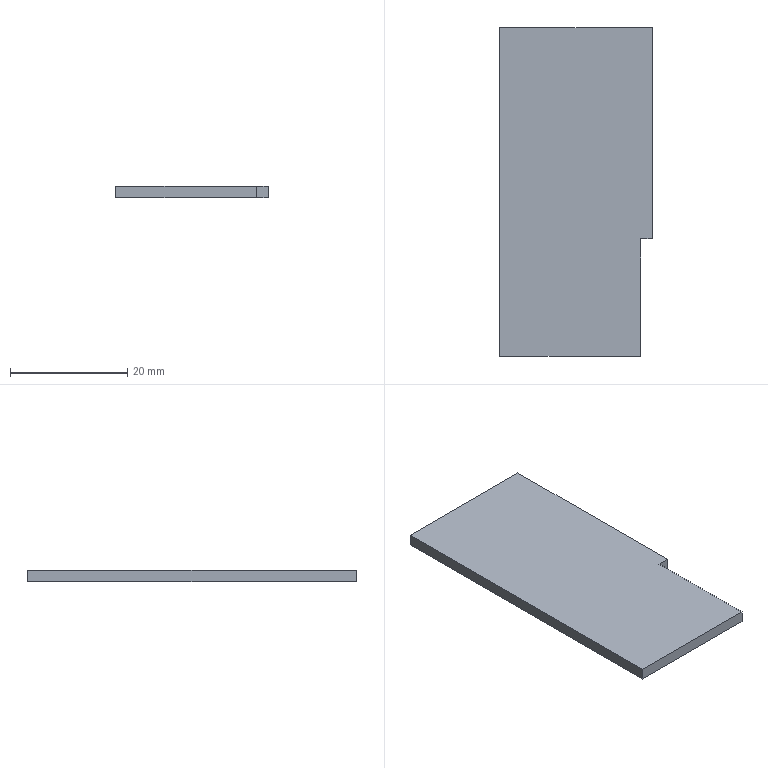Part | STEP file | Sliding Door Lower Rail Weldment-1 | 1 solid | 8 faces | box 26 x 56 x 2 mm | volume 2832 mm3 | plane 8
STEP:
#1=CARTESIAN_POINT('',(-7.603,-40.357,-2.));
#2=VERTEX_POINT('',#1);
#3=CARTESIAN_POINT('',(-7.603,-20.357,-2.));
#4=VERTEX_POINT('',#3);
#5=CARTESIAN_POINT('',(-7.603,0.,-2.));
#6=DIRECTION('',(0.,1.,0.));
#7=VECTOR('',#6,1000.);
#8=LINE('',#5,#7);
#9=EDGE_CURVE('',#2,#4,#8,.T.);
#10=ORIENTED_EDGE('',*,*,#9,.F.);
#11=CARTESIAN_POINT('',(-31.603,-40.357,-2.));
#12=VERTEX_POINT('',#11);
#13=CARTESIAN_POINT('',(0.,-40.357,-2.));
#14=DIRECTION('',(1.,0.,0.));
#15=VECTOR('',#14,1000.);
#16=LINE('',#13,#15);
#17=EDGE_CURVE('',#12,#2,#16,.T.);
#18=ORIENTED_EDGE('',*,*,#17,.F.);
#19=CARTESIAN_POINT('',(-31.603,15.643,-2.));
#20=VERTEX_POINT('',#19);
#21=CARTESIAN_POINT('',(-31.603,0.,-2.));
#22=DIRECTION('',(0.,-1.,0.));
#23=VECTOR('',#22,1000.);
#24=LINE('',#21,#23);
#25=EDGE_CURVE('',#20,#12,#24,.T.);
#26=ORIENTED_EDGE('',*,*,#25,.F.);
#27=CARTESIAN_POINT('',(-5.603,15.643,-2.));
#28=VERTEX_POINT('',#27);
#29=CARTESIAN_POINT('',(0.,15.643,-2.));
#30=DIRECTION('',(-1.,0.,0.));
#31=VECTOR('',#30,1000.);
#32=LINE('',#29,#31);
#33=EDGE_CURVE('',#28,#20,#32,.T.);
#34=ORIENTED_EDGE('',*,*,#33,.F.);
#35=CARTESIAN_POINT('',(-5.603,-20.357,-2.));
#36=VERTEX_POINT('',#35);
#37=CARTESIAN_POINT('',(-5.603,0.,-2.));
#38=DIRECTION('',(0.,1.,0.));
#39=VECTOR('',#38,1000.);
#40=LINE('',#37,#39);
#41=EDGE_CURVE('',#36,#28,#40,.T.);
#42=ORIENTED_EDGE('',*,*,#41,.F.);
#43=CARTESIAN_POINT('',(0.,-20.357,-2.));
#44=DIRECTION('',(1.,0.,0.));
#45=VECTOR('',#44,1000.);
#46=LINE('',#43,#45);
#47=EDGE_CURVE('',#4,#36,#46,.T.);
#48=ORIENTED_EDGE('',*,*,#47,.F.);
#49=EDGE_LOOP('',(#10,#18,#26,#34,#42,#48));
#50=FACE_OUTER_BOUND('',#49,.T.);
#51=CARTESIAN_POINT('',(0.,0.,-2.));
#52=DIRECTION('',(0.,0.,1.));
#53=DIRECTION('',(1.,0.,0.));
#54=AXIS2_PLACEMENT_3D('',#51,#52,#53);
#55=PLANE('',#54);
#56=ADVANCED_FACE('',(#50),#55,.F.);
#57=CARTESIAN_POINT('',(-7.603,-20.357,0.));
#58=VERTEX_POINT('',#57);
#59=CARTESIAN_POINT('',(-5.603,-20.357,0.));
#60=VERTEX_POINT('',#59);
#61=CARTESIAN_POINT('',(-5.603,-20.357,0.));
#62=DIRECTION('',(1.,0.,0.));
#63=VECTOR('',#62,1000.);
#64=LINE('',#61,#63);
#65=EDGE_CURVE('',#58,#60,#64,.T.);
#66=ORIENTED_EDGE('',*,*,#65,.F.);
#67=CARTESIAN_POINT('',(-7.603,-20.357,-10.));
#68=DIRECTION('',(0.,0.,1.));
#69=VECTOR('',#68,1000.);
#70=LINE('',#67,#69);
#71=EDGE_CURVE('',#4,#58,#70,.T.);
#72=ORIENTED_EDGE('',*,*,#71,.F.);
#73=ORIENTED_EDGE('',*,*,#47,.T.);
#74=CARTESIAN_POINT('',(-5.603,-20.357,-10.));
#75=DIRECTION('',(0.,0.,-1.));
#76=VECTOR('',#75,1000.);
#77=LINE('',#74,#76);
#78=EDGE_CURVE('',#60,#36,#77,.T.);
#79=ORIENTED_EDGE('',*,*,#78,.F.);
#80=EDGE_LOOP('',(#66,#72,#73,#79));
#81=FACE_OUTER_BOUND('',#80,.T.);
#82=CARTESIAN_POINT('',(-5.603,-20.357,-10.));
#83=DIRECTION('',(0.,1.,0.));
#84=DIRECTION('',(0.,0.,1.));
#85=AXIS2_PLACEMENT_3D('',#82,#83,#84);
#86=PLANE('',#85);
#87=ADVANCED_FACE('',(#81),#86,.F.);
#88=CARTESIAN_POINT('',(-7.603,-40.357,0.));
#89=VERTEX_POINT('',#88);
#90=CARTESIAN_POINT('',(-7.603,-40.357,0.));
#91=DIRECTION('',(0.,1.,0.));
#92=VECTOR('',#91,1000.);
#93=LINE('',#90,#92);
#94=EDGE_CURVE('',#89,#58,#93,.T.);
#95=ORIENTED_EDGE('',*,*,#94,.F.);
#96=CARTESIAN_POINT('',(-7.603,-40.357,-10.));
#97=DIRECTION('',(0.,0.,1.));
#98=VECTOR('',#97,1000.);
#99=LINE('',#96,#98);
#100=EDGE_CURVE('',#2,#89,#99,.T.);
#101=ORIENTED_EDGE('',*,*,#100,.F.);
#102=ORIENTED_EDGE('',*,*,#9,.T.);
#103=ORIENTED_EDGE('',*,*,#71,.T.);
#104=EDGE_LOOP('',(#95,#101,#102,#103));
#105=FACE_OUTER_BOUND('',#104,.T.);
#106=CARTESIAN_POINT('',(-7.603,-40.357,-10.));
#107=DIRECTION('',(-1.,0.,0.));
#108=DIRECTION('',(0.,0.,1.));
#109=AXIS2_PLACEMENT_3D('',#106,#107,#108);
#110=PLANE('',#109);
#111=ADVANCED_FACE('',(#105),#110,.F.);
#112=CARTESIAN_POINT('',(-31.603,-40.357,0.));
#113=VERTEX_POINT('',#112);
#114=CARTESIAN_POINT('',(-31.603,-40.357,-2.));
#115=DIRECTION('',(0.,0.,-1.));
#116=VECTOR('',#115,1000.);
#117=LINE('',#114,#116);
#118=EDGE_CURVE('',#113,#12,#117,.T.);
#119=ORIENTED_EDGE('',*,*,#118,.T.);
#120=ORIENTED_EDGE('',*,*,#17,.T.);
#121=ORIENTED_EDGE('',*,*,#100,.T.);
#122=CARTESIAN_POINT('',(-31.603,-40.357,0.));
#123=DIRECTION('',(-1.,0.,0.));
#124=VECTOR('',#123,1000.);
#125=LINE('',#122,#124);
#126=EDGE_CURVE('',#89,#113,#125,.T.);
#127=ORIENTED_EDGE('',*,*,#126,.T.);
#128=EDGE_LOOP('',(#119,#120,#121,#127));
#129=FACE_OUTER_BOUND('',#128,.T.);
#130=CARTESIAN_POINT('',(-31.603,-40.357,-2.));
#131=DIRECTION('',(0.,-1.,0.));
#132=DIRECTION('',(0.,0.,-1.));
#133=AXIS2_PLACEMENT_3D('',#130,#131,#132);
#134=PLANE('',#133);
#135=ADVANCED_FACE('',(#129),#134,.T.);
#136=ORIENTED_EDGE('',*,*,#25,.T.);
#137=ORIENTED_EDGE('',*,*,#118,.F.);
#138=CARTESIAN_POINT('',(-31.603,15.643,0.));
#139=VERTEX_POINT('',#138);
#140=CARTESIAN_POINT('',(-31.603,15.643,0.));
#141=DIRECTION('',(0.,1.,0.));
#142=VECTOR('',#141,1000.);
#143=LINE('',#140,#142);
#144=EDGE_CURVE('',#113,#139,#143,.T.);
#145=ORIENTED_EDGE('',*,*,#144,.T.);
#146=CARTESIAN_POINT('',(-31.603,15.643,-2.));
#147=DIRECTION('',(0.,0.,-1.));
#148=VECTOR('',#147,1000.);
#149=LINE('',#146,#148);
#150=EDGE_CURVE('',#139,#20,#149,.T.);
#151=ORIENTED_EDGE('',*,*,#150,.T.);
#152=EDGE_LOOP('',(#136,#137,#145,#151));
#153=FACE_OUTER_BOUND('',#152,.T.);
#154=CARTESIAN_POINT('',(-31.603,15.643,-2.));
#155=DIRECTION('',(-1.,0.,0.));
#156=DIRECTION('',(0.,-1.,0.));
#157=AXIS2_PLACEMENT_3D('',#154,#155,#156);
#158=PLANE('',#157);
#159=ADVANCED_FACE('',(#153),#158,.T.);
#160=ORIENTED_EDGE('',*,*,#33,.T.);
#161=ORIENTED_EDGE('',*,*,#150,.F.);
#162=CARTESIAN_POINT('',(-5.603,15.643,0.));
#163=VERTEX_POINT('',#162);
#164=CARTESIAN_POINT('',(-31.603,15.643,0.));
#165=DIRECTION('',(1.,0.,0.));
#166=VECTOR('',#165,1000.);
#167=LINE('',#164,#166);
#168=EDGE_CURVE('',#139,#163,#167,.T.);
#169=ORIENTED_EDGE('',*,*,#168,.T.);
#170=CARTESIAN_POINT('',(-5.603,15.643,-2.));
#171=DIRECTION('',(0.,0.,-1.));
#172=VECTOR('',#171,1000.);
#173=LINE('',#170,#172);
#174=EDGE_CURVE('',#163,#28,#173,.T.);
#175=ORIENTED_EDGE('',*,*,#174,.T.);
#176=EDGE_LOOP('',(#160,#161,#169,#175));
#177=FACE_OUTER_BOUND('',#176,.T.);
#178=CARTESIAN_POINT('',(-31.603,15.643,-2.));
#179=DIRECTION('',(0.,1.,0.));
#180=DIRECTION('',(0.,0.,1.));
#181=AXIS2_PLACEMENT_3D('',#178,#179,#180);
#182=PLANE('',#181);
#183=ADVANCED_FACE('',(#177),#182,.T.);
#184=ORIENTED_EDGE('',*,*,#174,.F.);
#185=CARTESIAN_POINT('',(-5.603,15.643,0.));
#186=DIRECTION('',(0.,-1.,0.));
#187=VECTOR('',#186,1000.);
#188=LINE('',#185,#187);
#189=EDGE_CURVE('',#163,#60,#188,.T.);
#190=ORIENTED_EDGE('',*,*,#189,.T.);
#191=ORIENTED_EDGE('',*,*,#78,.T.);
#192=ORIENTED_EDGE('',*,*,#41,.T.);
#193=EDGE_LOOP('',(#184,#190,#191,#192));
#194=FACE_OUTER_BOUND('',#193,.T.);
#195=CARTESIAN_POINT('',(-5.603,15.643,-2.));
#196=DIRECTION('',(1.,0.,0.));
#197=DIRECTION('',(0.,1.,0.));
#198=AXIS2_PLACEMENT_3D('',#195,#196,#197);
#199=PLANE('',#198);
#200=ADVANCED_FACE('',(#194),#199,.T.);
#201=ORIENTED_EDGE('',*,*,#144,.F.);
#202=ORIENTED_EDGE('',*,*,#126,.F.);
#203=ORIENTED_EDGE('',*,*,#94,.T.);
#204=ORIENTED_EDGE('',*,*,#65,.T.);
#205=ORIENTED_EDGE('',*,*,#189,.F.);
#206=ORIENTED_EDGE('',*,*,#168,.F.);
#207=EDGE_LOOP('',(#201,#202,#203,#204,#205,#206));
#208=FACE_OUTER_BOUND('',#207,.T.);
#209=CARTESIAN_POINT('',(0.,0.,0.));
#210=DIRECTION('',(0.,0.,1.));
#211=DIRECTION('',(1.,0.,0.));
#212=AXIS2_PLACEMENT_3D('',#209,#210,#211);
#213=PLANE('',#212);
#214=ADVANCED_FACE('',(#208),#213,.T.);
#215=CLOSED_SHELL('',(#56,#87,#111,#135,#159,#183,#200,#214));
#216=MANIFOLD_SOLID_BREP('',#215);
#217=CARTESIAN_POINT('',(0.,0.,0.));
#218=DIRECTION('',(0.,0.,1.));
#219=DIRECTION('',(1.,0.,0.));
#220=AXIS2_PLACEMENT_3D('',#217,#218,#219);
#221=(LENGTH_UNIT()NAMED_UNIT(*)SI_UNIT(.MILLI.,.METRE.));
#222=UNCERTAINTY_MEASURE_WITH_UNIT(LENGTH_MEASURE(0.00001),#221,'','');
#223=(NAMED_UNIT(*)PLANE_ANGLE_UNIT()SI_UNIT($,.RADIAN.));
#224=(NAMED_UNIT(*)SI_UNIT($,.STERADIAN.)SOLID_ANGLE_UNIT());
#225=(GEOMETRIC_REPRESENTATION_CONTEXT(3)GLOBAL_UNCERTAINTY_ASSIGNED_CONTEXT((#222))GLOBAL_UNIT_ASSIGNED_CONTEXT((#221,#223,#224))REPRESENTATION_CONTEXT('',''));
#226=ADVANCED_BREP_SHAPE_REPRESENTATION('',(#216,#220),#225);